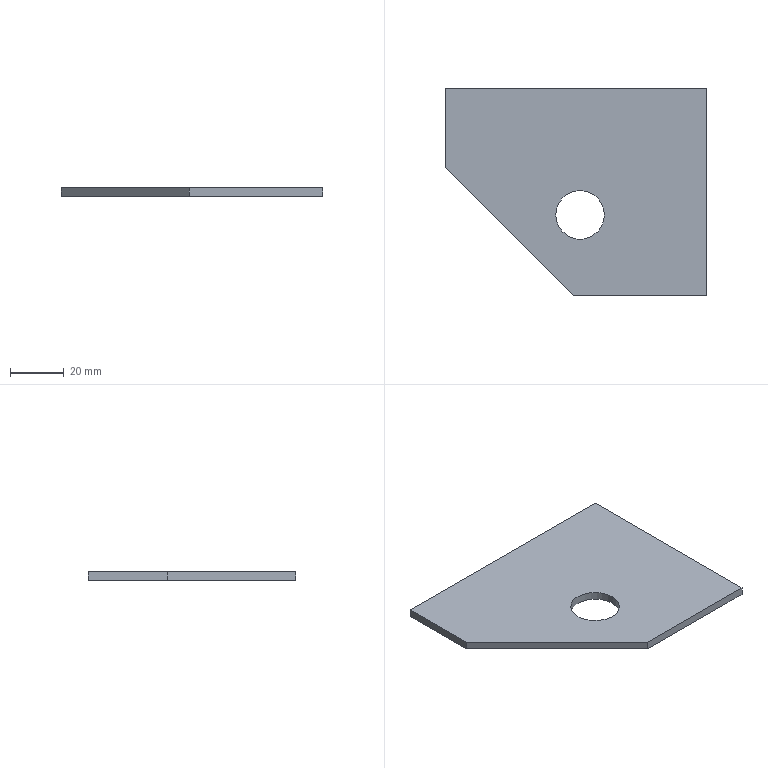Part | SolidWorks | features BaseBody 1 | 1 solid | 9 faces | box 97 x 77 x 3 mm | volume 18259 mm3 | plane 7 | cylinder 2 | commonest cylinder face diameters 18 x2
STEP:
#1=CARTESIAN_POINT('',(887.946,-3000.973,2112.471));
#2=VERTEX_POINT('',#1);
#3=CARTESIAN_POINT('',(905.946,-3000.973,2112.471));
#4=VERTEX_POINT('',#3);
#5=CARTESIAN_POINT('',(896.946,-3000.973,2112.471));
#6=DIRECTION('',(0.,0.,1.));
#7=DIRECTION('',(-1.,0.,0.));
#8=AXIS2_PLACEMENT_3D('',#5,#6,#7);
#9=CIRCLE('',#8,9.);
#10=EDGE_CURVE('',#2,#4,#9,.T.);
#11=ORIENTED_EDGE('',*,*,#10,.T.);
#12=CARTESIAN_POINT('',(905.946,-3000.973,2109.471));
#13=VERTEX_POINT('',#12);
#14=CARTESIAN_POINT('',(905.946,-3000.973,2112.471));
#15=DIRECTION('',(0.,0.,-1.));
#16=VECTOR('',#15,1000.);
#17=LINE('',#14,#16);
#18=EDGE_CURVE('',#4,#13,#17,.T.);
#19=ORIENTED_EDGE('',*,*,#18,.T.);
#20=CARTESIAN_POINT('',(887.946,-3000.973,2109.471));
#21=VERTEX_POINT('',#20);
#22=CARTESIAN_POINT('',(896.946,-3000.973,2109.471));
#23=DIRECTION('',(0.,0.,-1.));
#24=DIRECTION('',(-1.,0.,0.));
#25=AXIS2_PLACEMENT_3D('',#22,#23,#24);
#26=CIRCLE('',#25,9.);
#27=EDGE_CURVE('',#13,#21,#26,.T.);
#28=ORIENTED_EDGE('',*,*,#27,.T.);
#29=CARTESIAN_POINT('',(887.946,-3000.973,2112.471));
#30=DIRECTION('',(0.,0.,-1.));
#31=VECTOR('',#30,1000.);
#32=LINE('',#29,#31);
#33=EDGE_CURVE('',#2,#21,#32,.T.);
#34=ORIENTED_EDGE('',*,*,#33,.F.);
#35=EDGE_LOOP('',(#11,#19,#28,#34));
#36=FACE_OUTER_BOUND('',#35,.T.);
#37=CARTESIAN_POINT('',(896.946,-3000.973,2112.471));
#38=DIRECTION('',(0.,0.,-1.));
#39=DIRECTION('',(-1.,0.,0.));
#40=AXIS2_PLACEMENT_3D('',#37,#38,#39);
#41=CYLINDRICAL_SURFACE('',#40,9.);
#42=ADVANCED_FACE('',(#36),#41,.F.);
#43=CARTESIAN_POINT('',(846.946,-2983.473,2109.471));
#44=VERTEX_POINT('',#43);
#45=CARTESIAN_POINT('',(894.446,-3030.973,2109.471));
#46=VERTEX_POINT('',#45);
#47=CARTESIAN_POINT('',(846.946,-2983.473,2109.471));
#48=DIRECTION('',(0.7071,-0.7071,0.));
#49=VECTOR('',#48,1000.);
#50=LINE('',#47,#49);
#51=EDGE_CURVE('',#44,#46,#50,.T.);
#52=ORIENTED_EDGE('',*,*,#51,.F.);
#53=CARTESIAN_POINT('',(846.946,-2953.973,2109.471));
#54=VERTEX_POINT('',#53);
#55=CARTESIAN_POINT('',(846.946,-2994.262,2109.471));
#56=DIRECTION('',(0.,-1.,0.));
#57=VECTOR('',#56,1000.);
#58=LINE('',#55,#57);
#59=EDGE_CURVE('',#54,#44,#58,.T.);
#60=ORIENTED_EDGE('',*,*,#59,.F.);
#61=CARTESIAN_POINT('',(943.946,-2953.973,2109.471));
#62=VERTEX_POINT('',#61);
#63=CARTESIAN_POINT('',(903.657,-2953.973,2109.471));
#64=DIRECTION('',(-1.,0.,0.));
#65=VECTOR('',#64,1000.);
#66=LINE('',#63,#65);
#67=EDGE_CURVE('',#62,#54,#66,.T.);
#68=ORIENTED_EDGE('',*,*,#67,.F.);
#69=CARTESIAN_POINT('',(943.946,-3030.973,2109.471));
#70=VERTEX_POINT('',#69);
#71=CARTESIAN_POINT('',(943.946,-2994.262,2109.471));
#72=DIRECTION('',(0.,1.,0.));
#73=VECTOR('',#72,1000.);
#74=LINE('',#71,#73);
#75=EDGE_CURVE('',#70,#62,#74,.T.);
#76=ORIENTED_EDGE('',*,*,#75,.F.);
#77=CARTESIAN_POINT('',(903.657,-3030.973,2109.471));
#78=DIRECTION('',(1.,0.,0.));
#79=VECTOR('',#78,1000.);
#80=LINE('',#77,#79);
#81=EDGE_CURVE('',#46,#70,#80,.T.);
#82=ORIENTED_EDGE('',*,*,#81,.F.);
#83=EDGE_LOOP('',(#52,#60,#68,#76,#82));
#84=FACE_OUTER_BOUND('',#83,.T.);
#85=CARTESIAN_POINT('',(896.946,-3000.973,2109.471));
#86=DIRECTION('',(0.,0.,-1.));
#87=DIRECTION('',(-1.,0.,0.));
#88=AXIS2_PLACEMENT_3D('',#85,#86,#87);
#89=CIRCLE('',#88,9.);
#90=EDGE_CURVE('',#21,#13,#89,.T.);
#91=ORIENTED_EDGE('',*,*,#90,.F.);
#92=ORIENTED_EDGE('',*,*,#27,.F.);
#93=EDGE_LOOP('',(#91,#92));
#94=FACE_BOUND('',#93,.T.);
#95=CARTESIAN_POINT('',(903.657,-2994.262,2109.471));
#96=DIRECTION('',(0.,0.,1.));
#97=DIRECTION('',(1.,0.,0.));
#98=AXIS2_PLACEMENT_3D('',#95,#96,#97);
#99=PLANE('',#98);
#100=ADVANCED_FACE('',(#84,#94),#99,.F.);
#101=ORIENTED_EDGE('',*,*,#81,.T.);
#102=CARTESIAN_POINT('',(943.946,-3030.973,2112.471));
#103=VERTEX_POINT('',#102);
#104=CARTESIAN_POINT('',(943.946,-3030.973,2109.471));
#105=DIRECTION('',(0.,0.,1.));
#106=VECTOR('',#105,1000.);
#107=LINE('',#104,#106);
#108=EDGE_CURVE('',#70,#103,#107,.T.);
#109=ORIENTED_EDGE('',*,*,#108,.T.);
#110=CARTESIAN_POINT('',(894.446,-3030.973,2112.471));
#111=VERTEX_POINT('',#110);
#112=CARTESIAN_POINT('',(914.446,-3030.973,2112.471));
#113=DIRECTION('',(-1.,0.,0.));
#114=VECTOR('',#113,1000.);
#115=LINE('',#112,#114);
#116=EDGE_CURVE('',#103,#111,#115,.T.);
#117=ORIENTED_EDGE('',*,*,#116,.T.);
#118=CARTESIAN_POINT('',(894.446,-3030.973,2109.471));
#119=DIRECTION('',(0.,0.,-1.));
#120=VECTOR('',#119,1000.);
#121=LINE('',#118,#120);
#122=EDGE_CURVE('',#111,#46,#121,.T.);
#123=ORIENTED_EDGE('',*,*,#122,.T.);
#124=EDGE_LOOP('',(#101,#109,#117,#123));
#125=FACE_OUTER_BOUND('',#124,.T.);
#126=CARTESIAN_POINT('',(914.446,-3030.973,2109.471));
#127=DIRECTION('',(0.,-1.,0.));
#128=DIRECTION('',(0.,0.,-1.));
#129=AXIS2_PLACEMENT_3D('',#126,#127,#128);
#130=PLANE('',#129);
#131=ADVANCED_FACE('',(#125),#130,.T.);
#132=ORIENTED_EDGE('',*,*,#51,.T.);
#133=ORIENTED_EDGE('',*,*,#122,.F.);
#134=CARTESIAN_POINT('',(846.946,-2983.473,2112.471));
#135=VERTEX_POINT('',#134);
#136=CARTESIAN_POINT('',(846.946,-2983.473,2112.471));
#137=DIRECTION('',(-0.7071,0.7071,0.));
#138=VECTOR('',#137,1000.);
#139=LINE('',#136,#138);
#140=EDGE_CURVE('',#111,#135,#139,.T.);
#141=ORIENTED_EDGE('',*,*,#140,.T.);
#142=CARTESIAN_POINT('',(846.946,-2983.473,2109.471));
#143=DIRECTION('',(0.,0.,-1.));
#144=VECTOR('',#143,1000.);
#145=LINE('',#142,#144);
#146=EDGE_CURVE('',#135,#44,#145,.T.);
#147=ORIENTED_EDGE('',*,*,#146,.T.);
#148=EDGE_LOOP('',(#132,#133,#141,#147));
#149=FACE_OUTER_BOUND('',#148,.T.);
#150=CARTESIAN_POINT('',(846.946,-2983.473,2109.471));
#151=DIRECTION('',(-0.7071,-0.7071,0.));
#152=DIRECTION('',(0.7071,-0.7071,0.));
#153=AXIS2_PLACEMENT_3D('',#150,#151,#152);
#154=PLANE('',#153);
#155=ADVANCED_FACE('',(#149),#154,.T.);
#156=ORIENTED_EDGE('',*,*,#59,.T.);
#157=ORIENTED_EDGE('',*,*,#146,.F.);
#158=CARTESIAN_POINT('',(846.946,-2953.973,2112.471));
#159=VERTEX_POINT('',#158);
#160=CARTESIAN_POINT('',(846.946,-2953.973,2112.471));
#161=DIRECTION('',(0.,1.,0.));
#162=VECTOR('',#161,1000.);
#163=LINE('',#160,#162);
#164=EDGE_CURVE('',#135,#159,#163,.T.);
#165=ORIENTED_EDGE('',*,*,#164,.T.);
#166=CARTESIAN_POINT('',(846.946,-2953.973,2109.471));
#167=DIRECTION('',(0.,0.,-1.));
#168=VECTOR('',#167,1000.);
#169=LINE('',#166,#168);
#170=EDGE_CURVE('',#159,#54,#169,.T.);
#171=ORIENTED_EDGE('',*,*,#170,.T.);
#172=EDGE_LOOP('',(#156,#157,#165,#171));
#173=FACE_OUTER_BOUND('',#172,.T.);
#174=CARTESIAN_POINT('',(846.946,-2953.973,2109.471));
#175=DIRECTION('',(-1.,0.,0.));
#176=DIRECTION('',(0.,-1.,0.));
#177=AXIS2_PLACEMENT_3D('',#174,#175,#176);
#178=PLANE('',#177);
#179=ADVANCED_FACE('',(#173),#178,.T.);
#180=ORIENTED_EDGE('',*,*,#67,.T.);
#181=ORIENTED_EDGE('',*,*,#170,.F.);
#182=CARTESIAN_POINT('',(943.946,-2953.973,2112.471));
#183=VERTEX_POINT('',#182);
#184=CARTESIAN_POINT('',(943.946,-2953.973,2112.471));
#185=DIRECTION('',(1.,0.,0.));
#186=VECTOR('',#185,1000.);
#187=LINE('',#184,#186);
#188=EDGE_CURVE('',#159,#183,#187,.T.);
#189=ORIENTED_EDGE('',*,*,#188,.T.);
#190=CARTESIAN_POINT('',(943.946,-2953.973,2109.471));
#191=DIRECTION('',(0.,0.,-1.));
#192=VECTOR('',#191,1000.);
#193=LINE('',#190,#192);
#194=EDGE_CURVE('',#183,#62,#193,.T.);
#195=ORIENTED_EDGE('',*,*,#194,.T.);
#196=EDGE_LOOP('',(#180,#181,#189,#195));
#197=FACE_OUTER_BOUND('',#196,.T.);
#198=CARTESIAN_POINT('',(943.946,-2953.973,2109.471));
#199=DIRECTION('',(0.,1.,0.));
#200=DIRECTION('',(0.,0.,1.));
#201=AXIS2_PLACEMENT_3D('',#198,#199,#200);
#202=PLANE('',#201);
#203=ADVANCED_FACE('',(#197),#202,.T.);
#204=ORIENTED_EDGE('',*,*,#75,.T.);
#205=ORIENTED_EDGE('',*,*,#194,.F.);
#206=CARTESIAN_POINT('',(943.946,-3050.973,2112.471));
#207=DIRECTION('',(0.,-1.,0.));
#208=VECTOR('',#207,1000.);
#209=LINE('',#206,#208);
#210=EDGE_CURVE('',#183,#103,#209,.T.);
#211=ORIENTED_EDGE('',*,*,#210,.T.);
#212=ORIENTED_EDGE('',*,*,#108,.F.);
#213=EDGE_LOOP('',(#204,#205,#211,#212));
#214=FACE_OUTER_BOUND('',#213,.T.);
#215=CARTESIAN_POINT('',(943.946,-3050.973,2109.471));
#216=DIRECTION('',(1.,0.,0.));
#217=DIRECTION('',(0.,0.,-1.));
#218=AXIS2_PLACEMENT_3D('',#215,#216,#217);
#219=PLANE('',#218);
#220=ADVANCED_FACE('',(#214),#219,.T.);
#221=ORIENTED_EDGE('',*,*,#18,.F.);
#222=CARTESIAN_POINT('',(896.946,-3000.973,2112.471));
#223=DIRECTION('',(0.,0.,1.));
#224=DIRECTION('',(-1.,0.,0.));
#225=AXIS2_PLACEMENT_3D('',#222,#223,#224);
#226=CIRCLE('',#225,9.);
#227=EDGE_CURVE('',#4,#2,#226,.T.);
#228=ORIENTED_EDGE('',*,*,#227,.T.);
#229=ORIENTED_EDGE('',*,*,#33,.T.);
#230=ORIENTED_EDGE('',*,*,#90,.T.);
#231=EDGE_LOOP('',(#221,#228,#229,#230));
#232=FACE_OUTER_BOUND('',#231,.T.);
#233=CARTESIAN_POINT('',(896.946,-3000.973,2112.471));
#234=DIRECTION('',(0.,0.,-1.));
#235=DIRECTION('',(-1.,0.,0.));
#236=AXIS2_PLACEMENT_3D('',#233,#234,#235);
#237=CYLINDRICAL_SURFACE('',#236,9.);
#238=ADVANCED_FACE('',(#232),#237,.F.);
#239=ORIENTED_EDGE('',*,*,#140,.F.);
#240=ORIENTED_EDGE('',*,*,#116,.F.);
#241=ORIENTED_EDGE('',*,*,#210,.F.);
#242=ORIENTED_EDGE('',*,*,#188,.F.);
#243=ORIENTED_EDGE('',*,*,#164,.F.);
#244=EDGE_LOOP('',(#239,#240,#241,#242,#243));
#245=FACE_OUTER_BOUND('',#244,.T.);
#246=ORIENTED_EDGE('',*,*,#10,.F.);
#247=ORIENTED_EDGE('',*,*,#227,.F.);
#248=EDGE_LOOP('',(#246,#247));
#249=FACE_BOUND('',#248,.T.);
#250=CARTESIAN_POINT('',(903.657,-2974.262,2112.471));
#251=DIRECTION('',(0.,0.,1.));
#252=DIRECTION('',(1.,0.,0.));
#253=AXIS2_PLACEMENT_3D('',#250,#251,#252);
#254=PLANE('',#253);
#255=ADVANCED_FACE('',(#245,#249),#254,.T.);
#256=CLOSED_SHELL('',(#42,#100,#131,#155,#179,#203,#220,#238,#255));
#257=MANIFOLD_SOLID_BREP('',#256);
#258=CARTESIAN_POINT('',(0.,0.,0.));
#259=DIRECTION('',(0.,0.,1.));
#260=DIRECTION('',(1.,0.,0.));
#261=AXIS2_PLACEMENT_3D('',#258,#259,#260);
#262=(LENGTH_UNIT()NAMED_UNIT(*)SI_UNIT(.MILLI.,.METRE.));
#263=UNCERTAINTY_MEASURE_WITH_UNIT(LENGTH_MEASURE(0.00001),#262,'','');
#264=(NAMED_UNIT(*)PLANE_ANGLE_UNIT()SI_UNIT($,.RADIAN.));
#265=(NAMED_UNIT(*)SI_UNIT($,.STERADIAN.)SOLID_ANGLE_UNIT());
#266=(GEOMETRIC_REPRESENTATION_CONTEXT(3)GLOBAL_UNCERTAINTY_ASSIGNED_CONTEXT((#263))GLOBAL_UNIT_ASSIGNED_CONTEXT((#262,#264,#265))REPRESENTATION_CONTEXT('',''));
#267=ADVANCED_BREP_SHAPE_REPRESENTATION('',(#257,#261),#266);